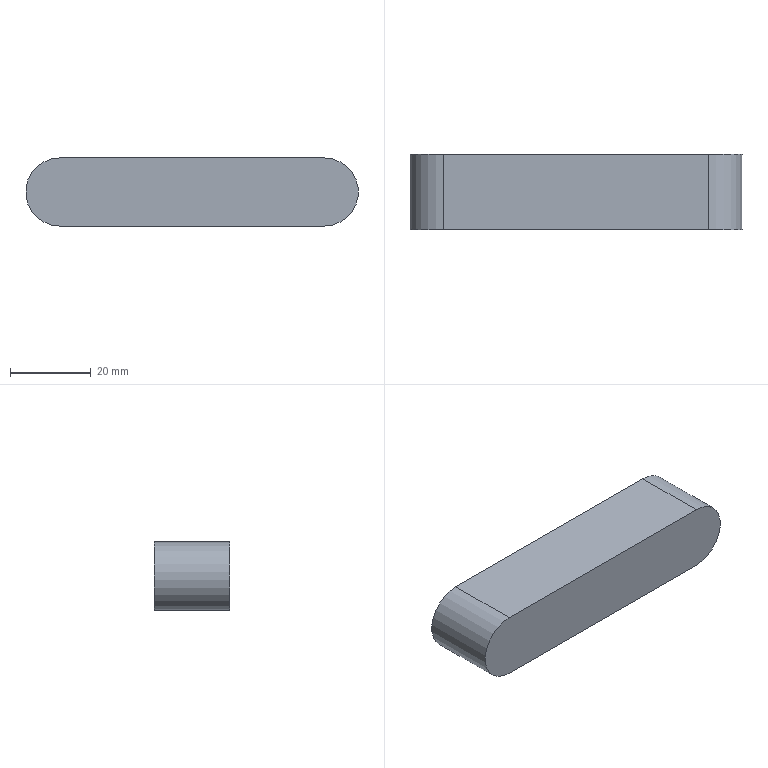Part | SolidWorks | features Extrusion 1, Scale 1 | 1 solid | 6 faces | box 82.5 x 18.75 x 16.875 mm | volume 24958 mm3 | plane 4 | cylinder 2 | commonest cylinder face diameters 16.875 x2
STEP:
#1=CARTESIAN_POINT('',(-15.313,-4.375,-8.437));
#2=VERTEX_POINT('',#1);
#3=CARTESIAN_POINT('',(-15.313,-4.375,8.437));
#4=VERTEX_POINT('',#3);
#5=CARTESIAN_POINT('',(-15.313,-4.375,0.));
#6=DIRECTION('',(0.,1.,0.));
#7=DIRECTION('',(0.,0.,1.));
#8=AXIS2_PLACEMENT_3D('',#5,#6,#7);
#9=CIRCLE('',#8,8.437);
#10=EDGE_CURVE('',#2,#4,#9,.T.);
#11=ORIENTED_EDGE('',*,*,#10,.T.);
#12=CARTESIAN_POINT('',(-15.313,14.375,8.437));
#13=VERTEX_POINT('',#12);
#14=CARTESIAN_POINT('',(-15.313,14.375,8.437));
#15=DIRECTION('',(0.,-1.,0.));
#16=VECTOR('',#15,1000.);
#17=LINE('',#14,#16);
#18=EDGE_CURVE('',#13,#4,#17,.T.);
#19=ORIENTED_EDGE('',*,*,#18,.F.);
#20=CARTESIAN_POINT('',(-15.313,14.375,-8.437));
#21=VERTEX_POINT('',#20);
#22=CARTESIAN_POINT('',(-15.313,14.375,0.));
#23=DIRECTION('',(0.,1.,0.));
#24=DIRECTION('',(0.,0.,1.));
#25=AXIS2_PLACEMENT_3D('',#22,#23,#24);
#26=CIRCLE('',#25,8.437);
#27=EDGE_CURVE('',#21,#13,#26,.T.);
#28=ORIENTED_EDGE('',*,*,#27,.F.);
#29=CARTESIAN_POINT('',(-15.313,14.375,-8.437));
#30=DIRECTION('',(0.,-1.,0.));
#31=VECTOR('',#30,1000.);
#32=LINE('',#29,#31);
#33=EDGE_CURVE('',#21,#2,#32,.T.);
#34=ORIENTED_EDGE('',*,*,#33,.T.);
#35=EDGE_LOOP('',(#11,#19,#28,#34));
#36=FACE_OUTER_BOUND('',#35,.T.);
#37=CARTESIAN_POINT('',(-15.313,14.375,0.));
#38=DIRECTION('',(0.,-1.,0.));
#39=DIRECTION('',(0.,0.,-1.));
#40=AXIS2_PLACEMENT_3D('',#37,#38,#39);
#41=CYLINDRICAL_SURFACE('',#40,8.437);
#42=ADVANCED_FACE('',(#36),#41,.T.);
#43=CARTESIAN_POINT('',(50.312,-4.375,8.437));
#44=VERTEX_POINT('',#43);
#45=CARTESIAN_POINT('',(-15.313,-4.375,8.437));
#46=DIRECTION('',(1.,0.,0.));
#47=VECTOR('',#46,1000.);
#48=LINE('',#45,#47);
#49=EDGE_CURVE('',#4,#44,#48,.T.);
#50=ORIENTED_EDGE('',*,*,#49,.T.);
#51=CARTESIAN_POINT('',(50.312,14.375,8.437));
#52=VERTEX_POINT('',#51);
#53=CARTESIAN_POINT('',(50.312,14.375,8.437));
#54=DIRECTION('',(0.,-1.,0.));
#55=VECTOR('',#54,1000.);
#56=LINE('',#53,#55);
#57=EDGE_CURVE('',#52,#44,#56,.T.);
#58=ORIENTED_EDGE('',*,*,#57,.F.);
#59=CARTESIAN_POINT('',(-15.313,14.375,8.437));
#60=DIRECTION('',(1.,0.,0.));
#61=VECTOR('',#60,1000.);
#62=LINE('',#59,#61);
#63=EDGE_CURVE('',#13,#52,#62,.T.);
#64=ORIENTED_EDGE('',*,*,#63,.F.);
#65=ORIENTED_EDGE('',*,*,#18,.T.);
#66=EDGE_LOOP('',(#50,#58,#64,#65));
#67=FACE_OUTER_BOUND('',#66,.T.);
#68=CARTESIAN_POINT('',(-15.313,14.375,8.437));
#69=DIRECTION('',(0.,0.,-1.));
#70=DIRECTION('',(-1.,0.,0.));
#71=AXIS2_PLACEMENT_3D('',#68,#69,#70);
#72=PLANE('',#71);
#73=ADVANCED_FACE('',(#67),#72,.F.);
#74=CARTESIAN_POINT('',(50.312,-4.375,-8.437));
#75=VERTEX_POINT('',#74);
#76=CARTESIAN_POINT('',(50.312,-4.375,0.));
#77=DIRECTION('',(0.,1.,0.));
#78=DIRECTION('',(0.,0.,1.));
#79=AXIS2_PLACEMENT_3D('',#76,#77,#78);
#80=CIRCLE('',#79,8.437);
#81=EDGE_CURVE('',#44,#75,#80,.T.);
#82=ORIENTED_EDGE('',*,*,#81,.T.);
#83=CARTESIAN_POINT('',(50.312,14.375,-8.437));
#84=VERTEX_POINT('',#83);
#85=CARTESIAN_POINT('',(50.312,14.375,-8.437));
#86=DIRECTION('',(0.,-1.,0.));
#87=VECTOR('',#86,1000.);
#88=LINE('',#85,#87);
#89=EDGE_CURVE('',#84,#75,#88,.T.);
#90=ORIENTED_EDGE('',*,*,#89,.F.);
#91=CARTESIAN_POINT('',(50.312,14.375,0.));
#92=DIRECTION('',(0.,1.,0.));
#93=DIRECTION('',(0.,0.,1.));
#94=AXIS2_PLACEMENT_3D('',#91,#92,#93);
#95=CIRCLE('',#94,8.437);
#96=EDGE_CURVE('',#52,#84,#95,.T.);
#97=ORIENTED_EDGE('',*,*,#96,.F.);
#98=ORIENTED_EDGE('',*,*,#57,.T.);
#99=EDGE_LOOP('',(#82,#90,#97,#98));
#100=FACE_OUTER_BOUND('',#99,.T.);
#101=CARTESIAN_POINT('',(50.312,14.375,0.));
#102=DIRECTION('',(0.,-1.,0.));
#103=DIRECTION('',(0.,0.,-1.));
#104=AXIS2_PLACEMENT_3D('',#101,#102,#103);
#105=CYLINDRICAL_SURFACE('',#104,8.437);
#106=ADVANCED_FACE('',(#100),#105,.T.);
#107=CARTESIAN_POINT('',(-15.313,-4.375,-8.437));
#108=DIRECTION('',(-1.,0.,0.));
#109=VECTOR('',#108,1000.);
#110=LINE('',#107,#109);
#111=EDGE_CURVE('',#75,#2,#110,.T.);
#112=ORIENTED_EDGE('',*,*,#111,.T.);
#113=ORIENTED_EDGE('',*,*,#33,.F.);
#114=CARTESIAN_POINT('',(-15.313,14.375,-8.437));
#115=DIRECTION('',(-1.,0.,0.));
#116=VECTOR('',#115,1000.);
#117=LINE('',#114,#116);
#118=EDGE_CURVE('',#84,#21,#117,.T.);
#119=ORIENTED_EDGE('',*,*,#118,.F.);
#120=ORIENTED_EDGE('',*,*,#89,.T.);
#121=EDGE_LOOP('',(#112,#113,#119,#120));
#122=FACE_OUTER_BOUND('',#121,.T.);
#123=CARTESIAN_POINT('',(-15.313,14.375,-8.437));
#124=DIRECTION('',(0.,0.,1.));
#125=DIRECTION('',(1.,0.,0.));
#126=AXIS2_PLACEMENT_3D('',#123,#124,#125);
#127=PLANE('',#126);
#128=ADVANCED_FACE('',(#122),#127,.F.);
#129=ORIENTED_EDGE('',*,*,#27,.T.);
#130=ORIENTED_EDGE('',*,*,#63,.T.);
#131=ORIENTED_EDGE('',*,*,#96,.T.);
#132=ORIENTED_EDGE('',*,*,#118,.T.);
#133=EDGE_LOOP('',(#129,#130,#131,#132));
#134=FACE_OUTER_BOUND('',#133,.T.);
#135=CARTESIAN_POINT('',(-15.313,14.375,0.));
#136=DIRECTION('',(0.,1.,0.));
#137=DIRECTION('',(0.,0.,1.));
#138=AXIS2_PLACEMENT_3D('',#135,#136,#137);
#139=PLANE('',#138);
#140=ADVANCED_FACE('',(#134),#139,.T.);
#141=ORIENTED_EDGE('',*,*,#10,.F.);
#142=ORIENTED_EDGE('',*,*,#111,.F.);
#143=ORIENTED_EDGE('',*,*,#81,.F.);
#144=ORIENTED_EDGE('',*,*,#49,.F.);
#145=EDGE_LOOP('',(#141,#142,#143,#144));
#146=FACE_OUTER_BOUND('',#145,.T.);
#147=CARTESIAN_POINT('',(-15.313,-4.375,0.));
#148=DIRECTION('',(0.,1.,0.));
#149=DIRECTION('',(0.,0.,1.));
#150=AXIS2_PLACEMENT_3D('',#147,#148,#149);
#151=PLANE('',#150);
#152=ADVANCED_FACE('',(#146),#151,.F.);
#153=CLOSED_SHELL('',(#42,#73,#106,#128,#140,#152));
#154=MANIFOLD_SOLID_BREP('',#153);
#155=CARTESIAN_POINT('',(0.,0.,0.));
#156=DIRECTION('',(0.,0.,1.));
#157=DIRECTION('',(1.,0.,0.));
#158=AXIS2_PLACEMENT_3D('',#155,#156,#157);
#159=(LENGTH_UNIT()NAMED_UNIT(*)SI_UNIT(.MILLI.,.METRE.));
#160=UNCERTAINTY_MEASURE_WITH_UNIT(LENGTH_MEASURE(0.00001),#159,'','');
#161=(NAMED_UNIT(*)PLANE_ANGLE_UNIT()SI_UNIT($,.RADIAN.));
#162=(NAMED_UNIT(*)SI_UNIT($,.STERADIAN.)SOLID_ANGLE_UNIT());
#163=(GEOMETRIC_REPRESENTATION_CONTEXT(3)GLOBAL_UNCERTAINTY_ASSIGNED_CONTEXT((#160))GLOBAL_UNIT_ASSIGNED_CONTEXT((#159,#161,#162))REPRESENTATION_CONTEXT('',''));
#164=ADVANCED_BREP_SHAPE_REPRESENTATION('',(#154,#158),#163);